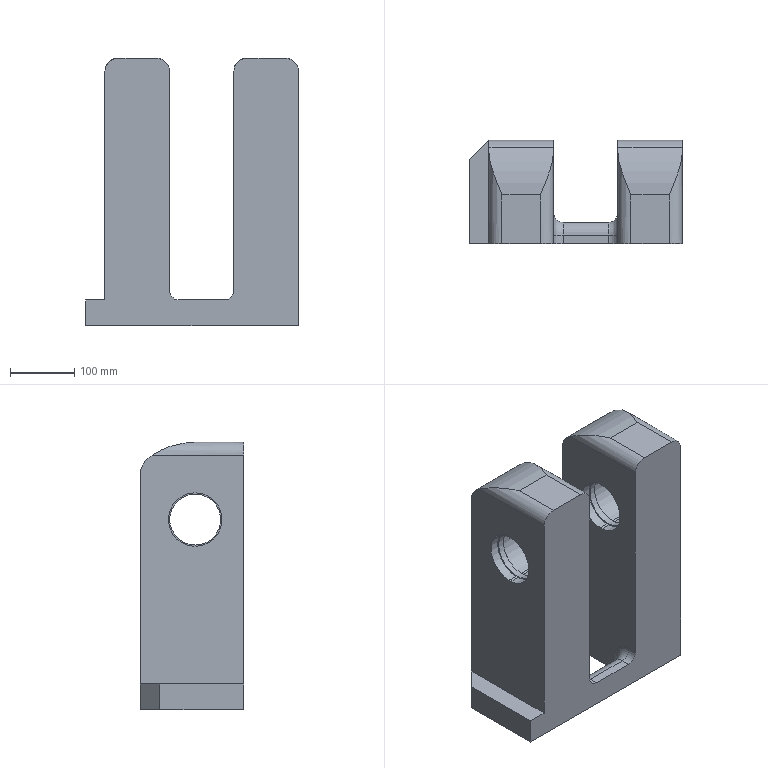Part | NX | features solid 2 | 1 solid | 83 faces | box 330 x 160 x 415 mm | volume 12290030 mm3 | plane 54 | cylinder 27 | torus 2 | commonest cylinder face diameters 83 x12 40 x5 79 x4 30 x2 60 x2 240 x2